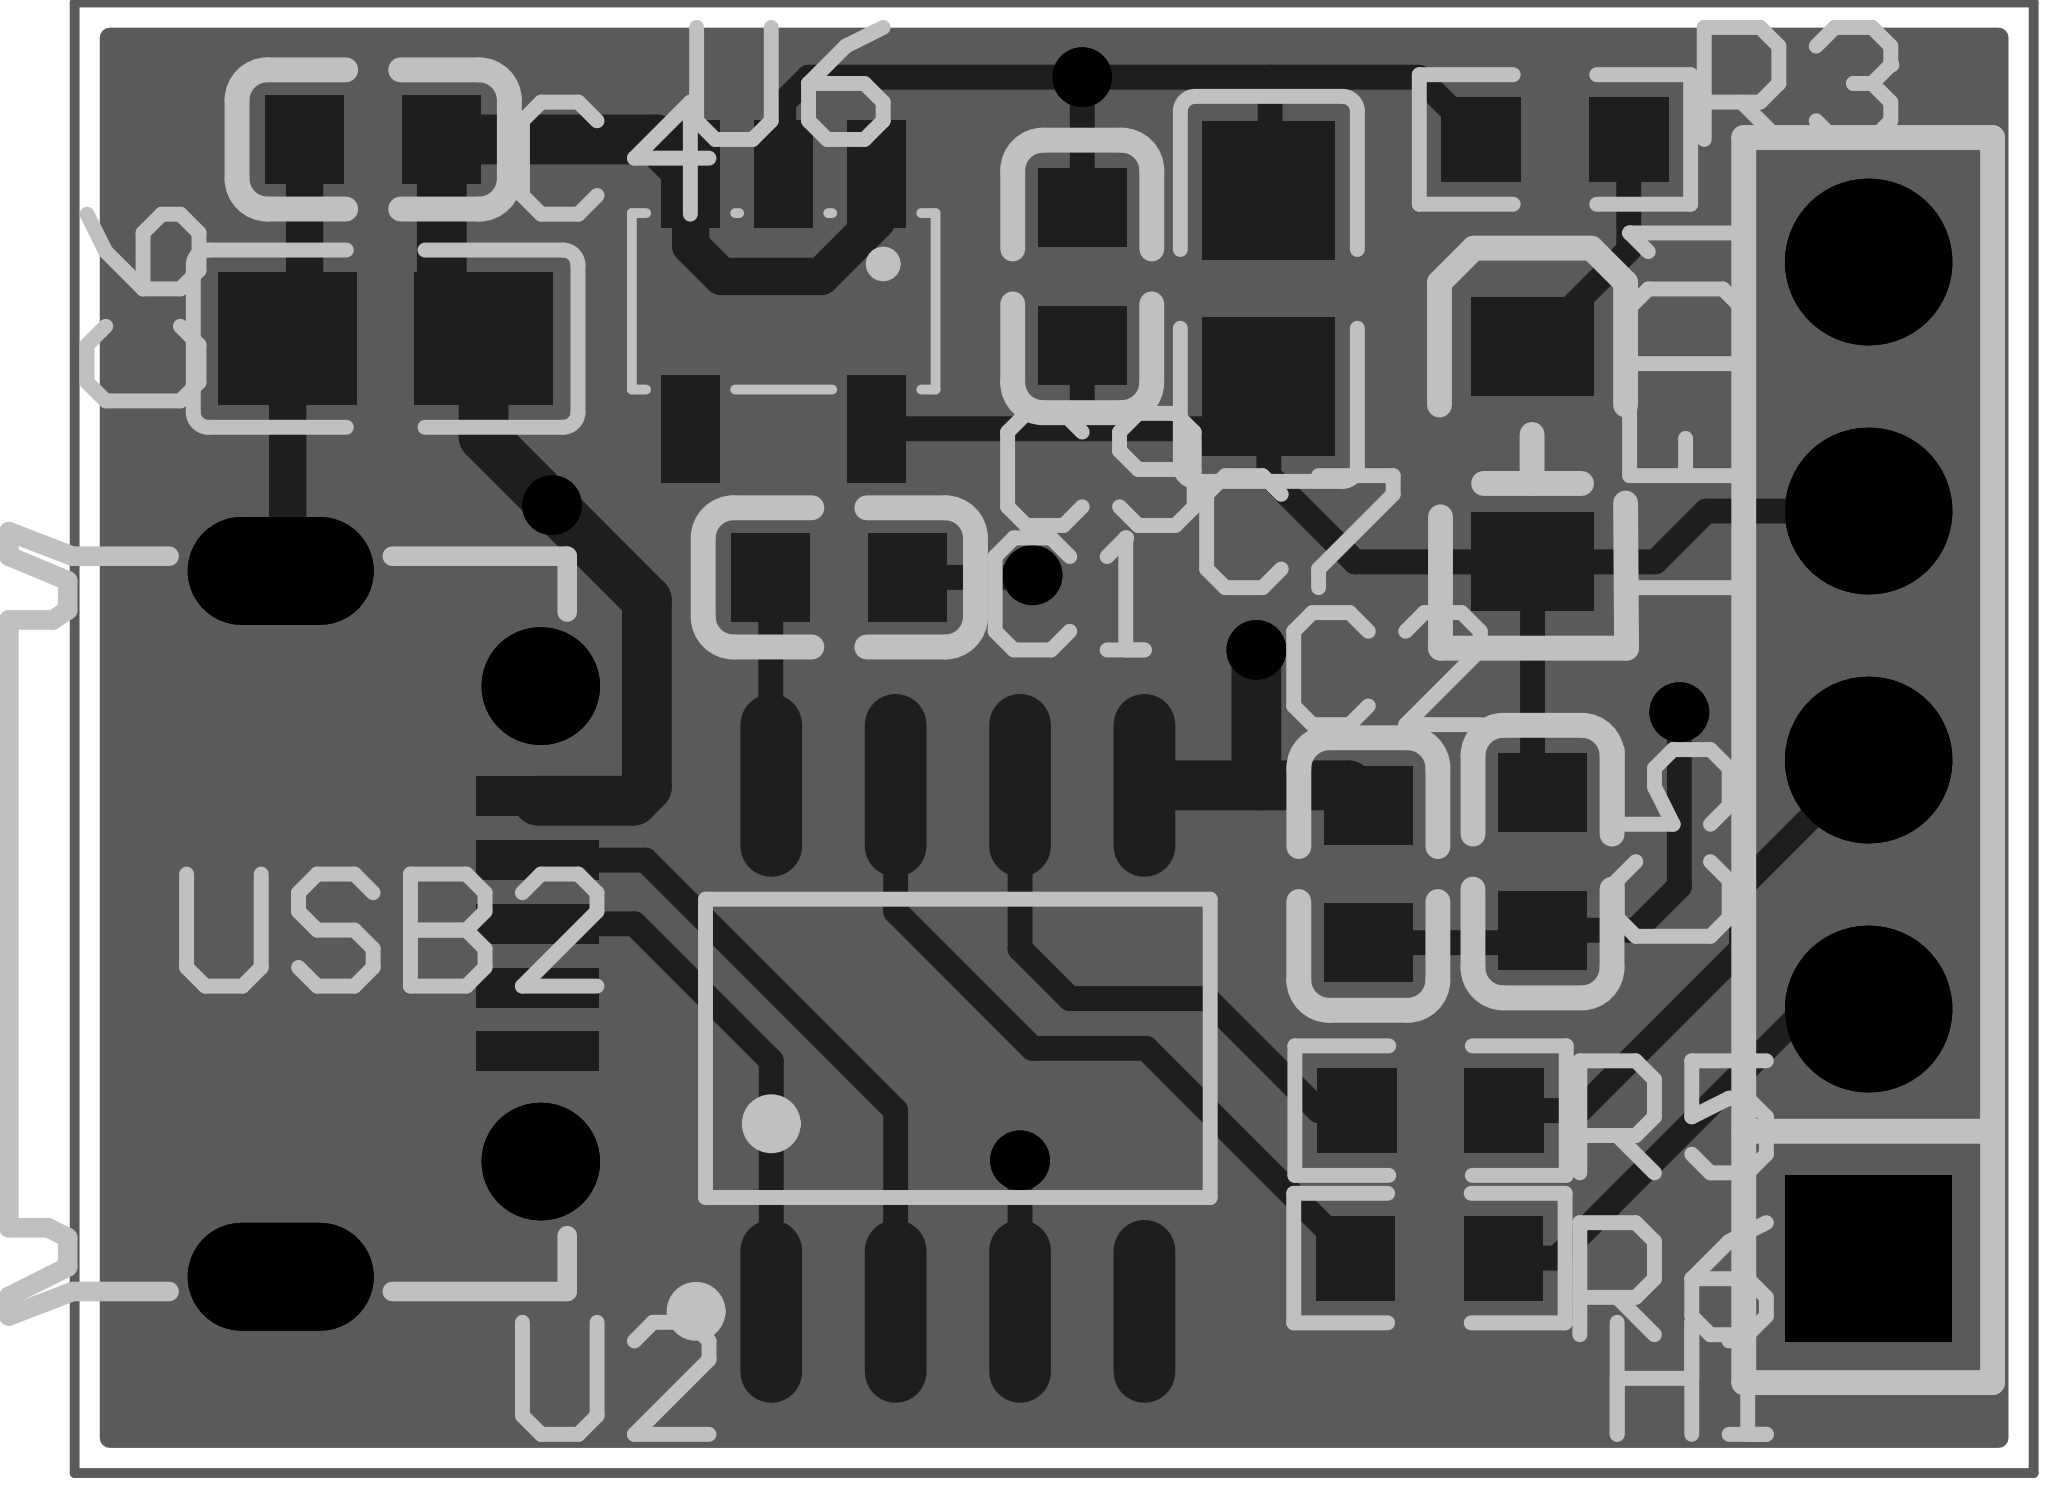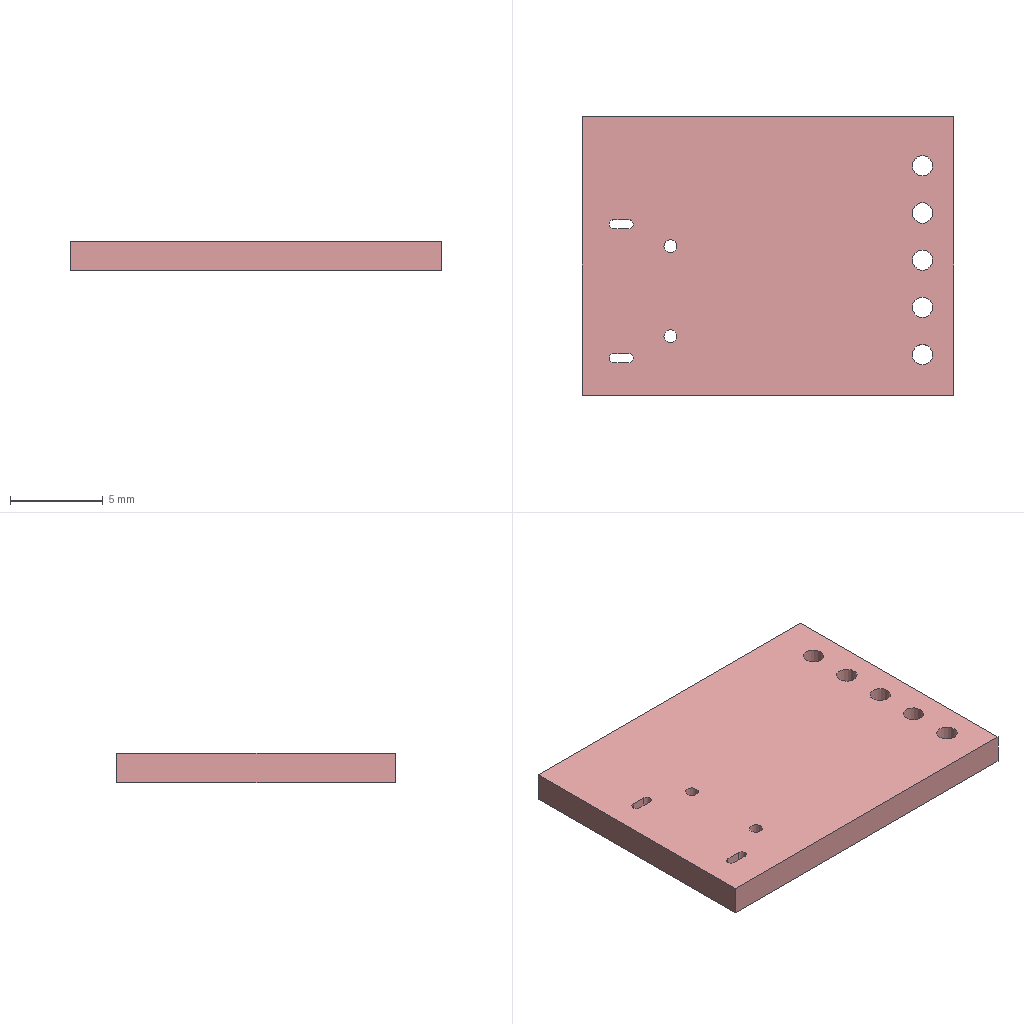Circuit board layout | Altium Designer | box 20 x 15 x 1.6 mm
Layer stack:
# Altium Designer layer stack of  (unit mm; dielectric type: 0 none, 1 core, 2 prepreg, 3 surface material)
index,name,kind,layer,copper_thickness_mm,dielectric_type,dielectric_thickness_mm,dielectric_material,dielectric_constant
0,Top Paste Mask Layer,other,,,,,,
1,Top Silkscreen Layer,other,,,,,,
2,Top Solder Mask Layer,dielectric,,,3,0.01,,3.3
3,Top Layer,copper,Top Layer,0.035,,,,
4,Dielectric1,dielectric,,,3,1.51,FR4,4.5
5,Bottom Layer,copper,Bottom Layer,0.035,,,,
6,Bottom Solder Mask Layer,dielectric,,,3,0.01,,3.3
7,Bottom Silkscreen Layer,other,,,,,,
8,Bottom Paste Mask Layer,other,,,,,,
# drill layer pairs: low layer,high layer
drill_pair,Top Layer,Bottom Layer
Part placement:
Designator,Comment,Layer,Footprint,Center-X(mm),Center-Y(mm),Rotation
C1,100nF,TopLayer,C0603,86.674,89.132,180
C2,100nF,TopLayer,C0603,92.075,86.106,90
C4,100nF,TopLayer,C0603,81.915,93.599,0
C5,100nF,TopLayer,C0603,93.853,86.233,90
C6,22uF,TopLayer,C0805,82.042,91.567,0
C7,22uF,TopLayer,C0805,91.059,92.075,270
C9,100nF,TopLayer,C0603,89.154,92.202,270
H1,PZ254V-11-05P,TopLayer,HDR-TH_5P-P2.54-V-M,97.178,87.269,90
LED1,NCD0805R1,TopLayer,LED0805-RD,93.751,90.39,270
R3,1kΩ,TopLayer,R0603,93.98,93.599,0
R5,22Ω,TopLayer,R0603,92.71,83.693,0
R6,22Ω,TopLayer,R0603,92.698,82.189,0
U2,CH340N,TopLayer,SOP-8_L4.9-W3.9-P1.27-LS6.0-BL,87.884,84.328,0
U6,XC6219B332MR,TopLayer,SOT-23-5_L3.0-W1.7-P0.95-LS2.8-BR,86.106,91.948,90
USB2,920-E52A2021S10100,TopLayer,MICRO-USB-SMD_5P-P0.65-H-F_C10418,82.296,85.598,270
Pad and via stacks:
# Altium Designer via and pad stacks of  (unit mm). Each distinct definition once, with the count of objects using it.
# via: kind,start_layer,end_layer,hole_mm,diameter_mm,mode(0 simple;1 top-mid-bottom;2 full stack),diameter_per_layer,count,example_net
# pad: kind,layer,hole_mm,hole_type(0 round;1 square;2 slot),plating,top_size,top_shape(1 round;2 rect;3 octagon;9 rounded rect),mid_size,bottom_size,mode,footprint,size_per_layer,count,example
pad,Top Layer,0,0,plated,0.8x0.9,2,0.8x0.9,0.8x0.9,0,C0603,,10,C1.2
pad,Top Layer,0,0,plated,1.41x1.35,2,1.41x1.35,1.41x1.35,0,C0805,,4,C6.2
pad,Top Layer,0,0,plated,1x1.25,2,1x1.25,1x1.25,0,LED0805-RD,,2,LED1.2
pad,Top Layer,0,0,plated,0.8065x0.864,2,0.8065x0.864,0.8065x0.864,0,R0603,,6,R3.2
pad,Top Layer,0,0,plated,0.63x1.865,1,0.63x1.865,0.63x1.865,0,SOP-8_L4.9-W3.9-P1.27-LS6.0-BL,,8,U2.1
pad,Top Layer,0,0,plated,1.1x0.6,2,1.1x0.6,1.1x0.6,0,SOT-23-5_L3.0-W1.7-P0.95-LS2.8-BR,,5,U6.5
pad,Top Layer,0,0,plated,1.25x0.4,2,1.25x0.4,1.25x0.4,0,MICRO-USB-SMD_5P-P0.65-H-F_C10418,,5,USB2.5
pad,Multi-Layer,1.1,0,plated,1.7x1.7,2,1.7x1.7,1.7x1.7,0,HDR-TH_5P-P2.54-V-M,,1,H1.1
pad,Multi-Layer,1.1,0,plated,1.7x1.7,1,1.7x1.7,1.7x1.7,0,HDR-TH_5P-P2.54-V-M,,4,H1.2
pad,Multi-Layer,0.5,2,plated,1.1x1.9,1,1.1x1.9,1.1x1.9,0,MICRO-USB-SMD_5P-P0.65-H-F_C10418,,2,USB2.SH2
pad,Multi-Layer,0.7,0,plated,1.2x1.2,1,1.2x1.2,1.2x1.2,0,MICRO-USB-SMD_5P-P0.65-H-F_C10418,,2,USB2.SH0
via,Top Layer,Bottom Layer,0.3048,0.61,0,,6,GND
Copper pours:
name,layer,net,type(0 solid;1 hatched;2 none)
Bottom Layer-GND,Bottom Layer,GND,0
Design rules, without the lines most boards share:
# Altium Designer design rules of  (exported by Altium Designer, unit mm)
# columns: name | kind | enabled | priority | scope1 | scope2 | descriptor | typed fields (field=value)
creepage | 65 | enabled | 1 | All | All | Creepage Distance Constraint =(0mil) (All),(All) |